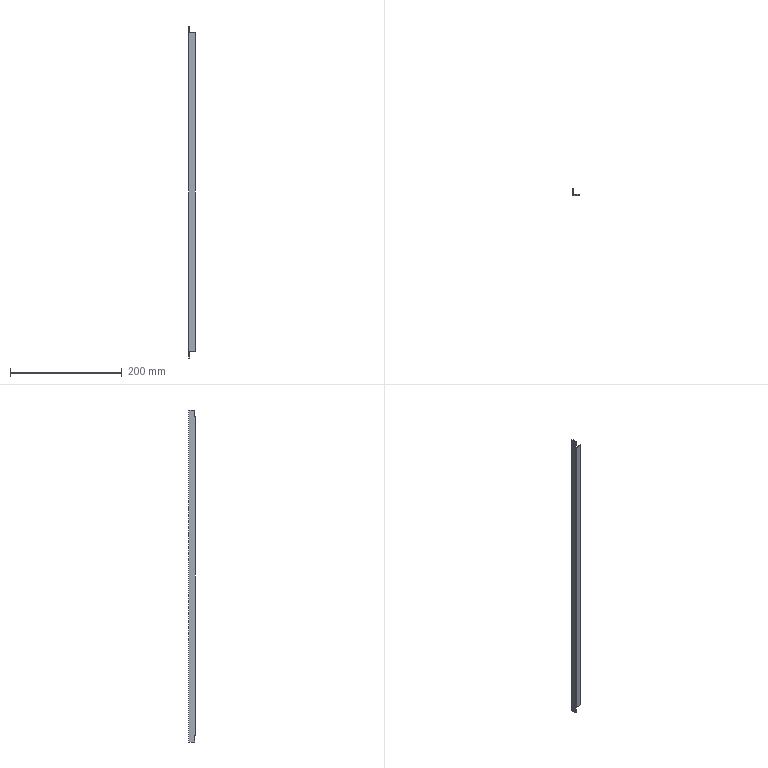Part | SolidWorks | features BaseBody 1 | 1 solid | 18 faces | box 12 x 12 x 594.4 mm | volume 15859 mm3 | plane 12 | cylinder 6 | commonest cylinder face diameters 0.6 x4 1 x2
STEP:
#1=CARTESIAN_POINT('',(0.,0.5,-284.7));
#2=VERTEX_POINT('',#1);
#3=CARTESIAN_POINT('',(0.5,0.,-284.7));
#4=VERTEX_POINT('',#3);
#5=CARTESIAN_POINT('',(0.5,0.5,-284.7));
#6=DIRECTION('',(0.,0.,1.));
#7=DIRECTION('',(-1.,0.,0.));
#8=AXIS2_PLACEMENT_3D('',#5,#6,#7);
#9=CIRCLE('',#8,0.5);
#10=EDGE_CURVE('',#2,#4,#9,.T.);
#11=ORIENTED_EDGE('',*,*,#10,.T.);
#12=CARTESIAN_POINT('',(0.5,0.,284.7));
#13=VERTEX_POINT('',#12);
#14=CARTESIAN_POINT('',(0.5,0.,0.));
#15=DIRECTION('',(0.,0.,-1.));
#16=VECTOR('',#15,1000.);
#17=LINE('',#14,#16);
#18=EDGE_CURVE('',#13,#4,#17,.T.);
#19=ORIENTED_EDGE('',*,*,#18,.F.);
#20=CARTESIAN_POINT('',(0.,0.5,284.7));
#21=VERTEX_POINT('',#20);
#22=CARTESIAN_POINT('',(0.5,0.5,284.7));
#23=DIRECTION('',(0.,0.,-1.));
#24=DIRECTION('',(-1.,0.,0.));
#25=AXIS2_PLACEMENT_3D('',#22,#23,#24);
#26=CIRCLE('',#25,0.5);
#27=EDGE_CURVE('',#13,#21,#26,.T.);
#28=ORIENTED_EDGE('',*,*,#27,.T.);
#29=CARTESIAN_POINT('',(0.,0.5,0.));
#30=DIRECTION('',(0.,0.,1.));
#31=VECTOR('',#30,1000.);
#32=LINE('',#29,#31);
#33=EDGE_CURVE('',#2,#21,#32,.T.);
#34=ORIENTED_EDGE('',*,*,#33,.F.);
#35=EDGE_LOOP('',(#11,#19,#28,#34));
#36=FACE_OUTER_BOUND('',#35,.T.);
#37=CARTESIAN_POINT('',(0.5,0.5,284.7));
#38=DIRECTION('',(0.,0.,-1.));
#39=DIRECTION('',(-1.,0.,0.));
#40=AXIS2_PLACEMENT_3D('',#37,#38,#39);
#41=CYLINDRICAL_SURFACE('',#40,0.5);
#42=ADVANCED_FACE('',(#36),#41,.T.);
#43=CARTESIAN_POINT('',(0.,1.2,-284.7));
#44=VERTEX_POINT('',#43);
#45=CARTESIAN_POINT('',(0.,0.6,-284.7));
#46=DIRECTION('',(0.,-1.,0.));
#47=VECTOR('',#46,1000.);
#48=LINE('',#45,#47);
#49=EDGE_CURVE('',#44,#2,#48,.T.);
#50=ORIENTED_EDGE('',*,*,#49,.T.);
#51=ORIENTED_EDGE('',*,*,#33,.T.);
#52=CARTESIAN_POINT('',(0.,1.2,284.7));
#53=VERTEX_POINT('',#52);
#54=CARTESIAN_POINT('',(0.,0.6,284.7));
#55=DIRECTION('',(0.,1.,0.));
#56=VECTOR('',#55,1000.);
#57=LINE('',#54,#56);
#58=EDGE_CURVE('',#21,#53,#57,.T.);
#59=ORIENTED_EDGE('',*,*,#58,.T.);
#60=CARTESIAN_POINT('',(0.,1.2,297.2));
#61=VERTEX_POINT('',#60);
#62=CARTESIAN_POINT('',(0.,1.2,0.));
#63=DIRECTION('',(0.,0.,-1.));
#64=VECTOR('',#63,1000.);
#65=LINE('',#62,#64);
#66=EDGE_CURVE('',#61,#53,#65,.T.);
#67=ORIENTED_EDGE('',*,*,#66,.F.);
#68=CARTESIAN_POINT('',(0.,11.7,297.2));
#69=VERTEX_POINT('',#68);
#70=CARTESIAN_POINT('',(0.,6.1,297.2));
#71=DIRECTION('',(0.,-1.,0.));
#72=VECTOR('',#71,1000.);
#73=LINE('',#70,#72);
#74=EDGE_CURVE('',#69,#61,#73,.T.);
#75=ORIENTED_EDGE('',*,*,#74,.F.);
#76=CARTESIAN_POINT('',(0.,11.7,-297.2));
#77=VERTEX_POINT('',#76);
#78=CARTESIAN_POINT('',(0.,11.7,0.));
#79=DIRECTION('',(0.,0.,1.));
#80=VECTOR('',#79,1000.);
#81=LINE('',#78,#80);
#82=EDGE_CURVE('',#77,#69,#81,.T.);
#83=ORIENTED_EDGE('',*,*,#82,.F.);
#84=CARTESIAN_POINT('',(0.,1.2,-297.2));
#85=VERTEX_POINT('',#84);
#86=CARTESIAN_POINT('',(0.,6.1,-297.2));
#87=DIRECTION('',(0.,1.,0.));
#88=VECTOR('',#87,1000.);
#89=LINE('',#86,#88);
#90=EDGE_CURVE('',#85,#77,#89,.T.);
#91=ORIENTED_EDGE('',*,*,#90,.F.);
#92=CARTESIAN_POINT('',(0.,1.2,0.));
#93=DIRECTION('',(0.,0.,-1.));
#94=VECTOR('',#93,1000.);
#95=LINE('',#92,#94);
#96=EDGE_CURVE('',#44,#85,#95,.T.);
#97=ORIENTED_EDGE('',*,*,#96,.F.);
#98=EDGE_LOOP('',(#50,#51,#59,#67,#75,#83,#91,#97));
#99=FACE_OUTER_BOUND('',#98,.T.);
#100=CARTESIAN_POINT('',(0.,0.5,297.2));
#101=DIRECTION('',(1.,0.,0.));
#102=DIRECTION('',(0.,0.,-1.));
#103=AXIS2_PLACEMENT_3D('',#100,#101,#102);
#104=PLANE('',#103);
#105=ADVANCED_FACE('',(#99),#104,.F.);
#106=CARTESIAN_POINT('',(11.7,0.,-284.7));
#107=VERTEX_POINT('',#106);
#108=CARTESIAN_POINT('',(6.1,0.,-284.7));
#109=DIRECTION('',(-1.,0.,0.));
#110=VECTOR('',#109,1000.);
#111=LINE('',#108,#110);
#112=EDGE_CURVE('',#107,#4,#111,.T.);
#113=ORIENTED_EDGE('',*,*,#112,.F.);
#114=CARTESIAN_POINT('',(11.7,0.,284.7));
#115=VERTEX_POINT('',#114);
#116=CARTESIAN_POINT('',(11.7,0.,0.));
#117=DIRECTION('',(0.,0.,-1.));
#118=VECTOR('',#117,1000.);
#119=LINE('',#116,#118);
#120=EDGE_CURVE('',#115,#107,#119,.T.);
#121=ORIENTED_EDGE('',*,*,#120,.F.);
#122=CARTESIAN_POINT('',(6.1,0.,284.7));
#123=DIRECTION('',(1.,0.,0.));
#124=VECTOR('',#123,1000.);
#125=LINE('',#122,#124);
#126=EDGE_CURVE('',#13,#115,#125,.T.);
#127=ORIENTED_EDGE('',*,*,#126,.F.);
#128=ORIENTED_EDGE('',*,*,#18,.T.);
#129=EDGE_LOOP('',(#113,#121,#127,#128));
#130=FACE_OUTER_BOUND('',#129,.T.);
#131=CARTESIAN_POINT('',(0.5,0.,-284.7));
#132=DIRECTION('',(0.,1.,0.));
#133=DIRECTION('',(0.,0.,1.));
#134=AXIS2_PLACEMENT_3D('',#131,#132,#133);
#135=PLANE('',#134);
#136=ADVANCED_FACE('',(#130),#135,.F.);
#137=CARTESIAN_POINT('',(1.7,1.2,-284.7));
#138=VERTEX_POINT('',#137);
#139=CARTESIAN_POINT('',(0.85,1.2,-284.7));
#140=DIRECTION('',(1.,0.,0.));
#141=VECTOR('',#140,1000.);
#142=LINE('',#139,#141);
#143=EDGE_CURVE('',#44,#138,#142,.T.);
#144=ORIENTED_EDGE('',*,*,#143,.F.);
#145=ORIENTED_EDGE('',*,*,#96,.T.);
#146=CARTESIAN_POINT('',(1.7,1.2,-297.2));
#147=VERTEX_POINT('',#146);
#148=CARTESIAN_POINT('',(0.85,1.2,-297.2));
#149=DIRECTION('',(-1.,0.,0.));
#150=VECTOR('',#149,1000.);
#151=LINE('',#148,#150);
#152=EDGE_CURVE('',#147,#85,#151,.T.);
#153=ORIENTED_EDGE('',*,*,#152,.F.);
#154=CARTESIAN_POINT('',(1.7,1.2,-290.95));
#155=DIRECTION('',(0.,0.,-1.));
#156=VECTOR('',#155,1000.);
#157=LINE('',#154,#156);
#158=EDGE_CURVE('',#138,#147,#157,.T.);
#159=ORIENTED_EDGE('',*,*,#158,.F.);
#160=EDGE_LOOP('',(#144,#145,#153,#159));
#161=FACE_OUTER_BOUND('',#160,.T.);
#162=CARTESIAN_POINT('',(0.,1.2,-297.2));
#163=DIRECTION('',(0.,1.,0.));
#164=DIRECTION('',(0.,0.,1.));
#165=AXIS2_PLACEMENT_3D('',#162,#163,#164);
#166=PLANE('',#165);
#167=ADVANCED_FACE('',(#161),#166,.F.);
#168=CARTESIAN_POINT('',(1.7,1.2,297.2));
#169=VERTEX_POINT('',#168);
#170=CARTESIAN_POINT('',(0.85,1.2,297.2));
#171=DIRECTION('',(1.,0.,0.));
#172=VECTOR('',#171,1000.);
#173=LINE('',#170,#172);
#174=EDGE_CURVE('',#61,#169,#173,.T.);
#175=ORIENTED_EDGE('',*,*,#174,.F.);
#176=ORIENTED_EDGE('',*,*,#66,.T.);
#177=CARTESIAN_POINT('',(1.7,1.2,284.7));
#178=VERTEX_POINT('',#177);
#179=CARTESIAN_POINT('',(0.85,1.2,284.7));
#180=DIRECTION('',(-1.,0.,0.));
#181=VECTOR('',#180,1000.);
#182=LINE('',#179,#181);
#183=EDGE_CURVE('',#178,#53,#182,.T.);
#184=ORIENTED_EDGE('',*,*,#183,.F.);
#185=CARTESIAN_POINT('',(1.7,1.2,290.95));
#186=DIRECTION('',(0.,0.,-1.));
#187=VECTOR('',#186,1000.);
#188=LINE('',#185,#187);
#189=EDGE_CURVE('',#169,#178,#188,.T.);
#190=ORIENTED_EDGE('',*,*,#189,.F.);
#191=EDGE_LOOP('',(#175,#176,#184,#190));
#192=FACE_OUTER_BOUND('',#191,.T.);
#193=CARTESIAN_POINT('',(0.,1.2,284.7));
#194=DIRECTION('',(0.,1.,0.));
#195=DIRECTION('',(0.,0.,1.));
#196=AXIS2_PLACEMENT_3D('',#193,#194,#195);
#197=PLANE('',#196);
#198=ADVANCED_FACE('',(#192),#197,.F.);
#199=ORIENTED_EDGE('',*,*,#174,.T.);
#200=CARTESIAN_POINT('',(1.2,1.7,297.2));
#201=VERTEX_POINT('',#200);
#202=CARTESIAN_POINT('',(1.7,1.7,297.2));
#203=DIRECTION('',(0.,0.,1.));
#204=DIRECTION('',(-1.,0.,0.));
#205=AXIS2_PLACEMENT_3D('',#202,#203,#204);
#206=CIRCLE('',#205,0.5);
#207=EDGE_CURVE('',#201,#169,#206,.T.);
#208=ORIENTED_EDGE('',*,*,#207,.F.);
#209=CARTESIAN_POINT('',(1.2,11.7,297.2));
#210=VERTEX_POINT('',#209);
#211=CARTESIAN_POINT('',(1.2,6.6,297.2));
#212=DIRECTION('',(0.,-1.,0.));
#213=VECTOR('',#212,1000.);
#214=LINE('',#211,#213);
#215=EDGE_CURVE('',#210,#201,#214,.T.);
#216=ORIENTED_EDGE('',*,*,#215,.F.);
#217=CARTESIAN_POINT('',(0.9,12.,297.2));
#218=VERTEX_POINT('',#217);
#219=CARTESIAN_POINT('',(0.9,11.7,297.2));
#220=DIRECTION('',(0.,0.,1.));
#221=DIRECTION('',(-1.,0.,0.));
#222=AXIS2_PLACEMENT_3D('',#219,#220,#221);
#223=CIRCLE('',#222,0.3);
#224=EDGE_CURVE('',#210,#218,#223,.T.);
#225=ORIENTED_EDGE('',*,*,#224,.T.);
#226=CARTESIAN_POINT('',(0.3,12.,297.2));
#227=VERTEX_POINT('',#226);
#228=CARTESIAN_POINT('',(0.6,12.,297.2));
#229=DIRECTION('',(-1.,0.,0.));
#230=VECTOR('',#229,1000.);
#231=LINE('',#228,#230);
#232=EDGE_CURVE('',#218,#227,#231,.T.);
#233=ORIENTED_EDGE('',*,*,#232,.T.);
#234=CARTESIAN_POINT('',(0.3,11.7,297.2));
#235=DIRECTION('',(0.,0.,-1.));
#236=DIRECTION('',(-1.,0.,0.));
#237=AXIS2_PLACEMENT_3D('',#234,#235,#236);
#238=CIRCLE('',#237,0.3);
#239=EDGE_CURVE('',#69,#227,#238,.T.);
#240=ORIENTED_EDGE('',*,*,#239,.F.);
#241=ORIENTED_EDGE('',*,*,#74,.T.);
#242=EDGE_LOOP('',(#199,#208,#216,#225,#233,#240,#241));
#243=FACE_OUTER_BOUND('',#242,.T.);
#244=CARTESIAN_POINT('',(1.71,1.2,297.2));
#245=DIRECTION('',(0.,0.,-1.));
#246=DIRECTION('',(-1.,0.,0.));
#247=AXIS2_PLACEMENT_3D('',#244,#245,#246);
#248=PLANE('',#247);
#249=ADVANCED_FACE('',(#243),#248,.F.);
#250=ORIENTED_EDGE('',*,*,#82,.T.);
#251=ORIENTED_EDGE('',*,*,#239,.T.);
#252=CARTESIAN_POINT('',(0.3,12.,-297.2));
#253=VERTEX_POINT('',#252);
#254=CARTESIAN_POINT('',(0.3,12.,0.));
#255=DIRECTION('',(0.,0.,1.));
#256=VECTOR('',#255,1000.);
#257=LINE('',#254,#256);
#258=EDGE_CURVE('',#253,#227,#257,.T.);
#259=ORIENTED_EDGE('',*,*,#258,.F.);
#260=CARTESIAN_POINT('',(0.3,11.7,-297.2));
#261=DIRECTION('',(0.,0.,-1.));
#262=DIRECTION('',(-1.,0.,0.));
#263=AXIS2_PLACEMENT_3D('',#260,#261,#262);
#264=CIRCLE('',#263,0.3);
#265=EDGE_CURVE('',#77,#253,#264,.T.);
#266=ORIENTED_EDGE('',*,*,#265,.F.);
#267=EDGE_LOOP('',(#250,#251,#259,#266));
#268=FACE_OUTER_BOUND('',#267,.T.);
#269=CARTESIAN_POINT('',(0.3,11.7,297.2));
#270=DIRECTION('',(0.,0.,-1.));
#271=DIRECTION('',(-1.,0.,0.));
#272=AXIS2_PLACEMENT_3D('',#269,#270,#271);
#273=CYLINDRICAL_SURFACE('',#272,0.3);
#274=ADVANCED_FACE('',(#268),#273,.T.);
#275=CARTESIAN_POINT('',(1.2,11.7,-297.2));
#276=VERTEX_POINT('',#275);
#277=CARTESIAN_POINT('',(1.2,1.7,-297.2));
#278=VERTEX_POINT('',#277);
#279=CARTESIAN_POINT('',(1.2,6.6,-297.2));
#280=DIRECTION('',(0.,-1.,0.));
#281=VECTOR('',#280,1000.);
#282=LINE('',#279,#281);
#283=EDGE_CURVE('',#276,#278,#282,.T.);
#284=ORIENTED_EDGE('',*,*,#283,.T.);
#285=CARTESIAN_POINT('',(1.7,1.7,-297.2));
#286=DIRECTION('',(0.,0.,1.));
#287=DIRECTION('',(-1.,0.,0.));
#288=AXIS2_PLACEMENT_3D('',#285,#286,#287);
#289=CIRCLE('',#288,0.5);
#290=EDGE_CURVE('',#278,#147,#289,.T.);
#291=ORIENTED_EDGE('',*,*,#290,.T.);
#292=ORIENTED_EDGE('',*,*,#152,.T.);
#293=ORIENTED_EDGE('',*,*,#90,.T.);
#294=ORIENTED_EDGE('',*,*,#265,.T.);
#295=CARTESIAN_POINT('',(0.9,12.,-297.2));
#296=VERTEX_POINT('',#295);
#297=CARTESIAN_POINT('',(0.8551,12.,-297.2));
#298=DIRECTION('',(1.,0.,0.));
#299=VECTOR('',#298,1000.);
#300=LINE('',#297,#299);
#301=EDGE_CURVE('',#253,#296,#300,.T.);
#302=ORIENTED_EDGE('',*,*,#301,.T.);
#303=CARTESIAN_POINT('',(0.9,11.7,-297.2));
#304=DIRECTION('',(0.,0.,-1.));
#305=DIRECTION('',(-1.,0.,0.));
#306=AXIS2_PLACEMENT_3D('',#303,#304,#305);
#307=CIRCLE('',#306,0.3);
#308=EDGE_CURVE('',#296,#276,#307,.T.);
#309=ORIENTED_EDGE('',*,*,#308,.T.);
#310=EDGE_LOOP('',(#284,#291,#292,#293,#294,#302,#309));
#311=FACE_OUTER_BOUND('',#310,.T.);
#312=CARTESIAN_POINT('',(1.71,1.2,-297.2));
#313=DIRECTION('',(0.,0.,-1.));
#314=DIRECTION('',(-1.,0.,0.));
#315=AXIS2_PLACEMENT_3D('',#312,#313,#314);
#316=PLANE('',#315);
#317=ADVANCED_FACE('',(#311),#316,.T.);
#318=ORIENTED_EDGE('',*,*,#10,.F.);
#319=ORIENTED_EDGE('',*,*,#49,.F.);
#320=ORIENTED_EDGE('',*,*,#143,.T.);
#321=CARTESIAN_POINT('',(11.7,1.2,-284.7));
#322=VERTEX_POINT('',#321);
#323=CARTESIAN_POINT('',(6.,1.2,-284.7));
#324=DIRECTION('',(-1.,0.,0.));
#325=VECTOR('',#324,1000.);
#326=LINE('',#323,#325);
#327=EDGE_CURVE('',#322,#138,#326,.T.);
#328=ORIENTED_EDGE('',*,*,#327,.F.);
#329=CARTESIAN_POINT('',(12.,0.9,-284.7));
#330=VERTEX_POINT('',#329);
#331=CARTESIAN_POINT('',(11.7,0.9,-284.7));
#332=DIRECTION('',(0.,0.,-1.));
#333=DIRECTION('',(-1.,0.,0.));
#334=AXIS2_PLACEMENT_3D('',#331,#332,#333);
#335=CIRCLE('',#334,0.3);
#336=EDGE_CURVE('',#322,#330,#335,.T.);
#337=ORIENTED_EDGE('',*,*,#336,.T.);
#338=CARTESIAN_POINT('',(12.,0.3,-284.7));
#339=VERTEX_POINT('',#338);
#340=CARTESIAN_POINT('',(12.,0.6,-284.7));
#341=DIRECTION('',(0.,-1.,0.));
#342=VECTOR('',#341,1000.);
#343=LINE('',#340,#342);
#344=EDGE_CURVE('',#330,#339,#343,.T.);
#345=ORIENTED_EDGE('',*,*,#344,.T.);
#346=CARTESIAN_POINT('',(11.7,0.3,-284.7));
#347=DIRECTION('',(0.,0.,1.));
#348=DIRECTION('',(-1.,0.,0.));
#349=AXIS2_PLACEMENT_3D('',#346,#347,#348);
#350=CIRCLE('',#349,0.3);
#351=EDGE_CURVE('',#107,#339,#350,.T.);
#352=ORIENTED_EDGE('',*,*,#351,.F.);
#353=ORIENTED_EDGE('',*,*,#112,.T.);
#354=EDGE_LOOP('',(#318,#319,#320,#328,#337,#345,#352,#353));
#355=FACE_OUTER_BOUND('',#354,.T.);
#356=CARTESIAN_POINT('',(0.,1.2,-284.7));
#357=DIRECTION('',(0.,0.,1.));
#358=DIRECTION('',(0.,-1.,0.));
#359=AXIS2_PLACEMENT_3D('',#356,#357,#358);
#360=PLANE('',#359);
#361=ADVANCED_FACE('',(#355),#360,.F.);
#362=ORIENTED_EDGE('',*,*,#351,.T.);
#363=CARTESIAN_POINT('',(12.,0.3,284.7));
#364=VERTEX_POINT('',#363);
#365=CARTESIAN_POINT('',(12.,0.3,0.));
#366=DIRECTION('',(0.,0.,-1.));
#367=VECTOR('',#366,1000.);
#368=LINE('',#365,#367);
#369=EDGE_CURVE('',#364,#339,#368,.T.);
#370=ORIENTED_EDGE('',*,*,#369,.F.);
#371=CARTESIAN_POINT('',(11.7,0.3,284.7));
#372=DIRECTION('',(0.,0.,1.));
#373=DIRECTION('',(-1.,0.,0.));
#374=AXIS2_PLACEMENT_3D('',#371,#372,#373);
#375=CIRCLE('',#374,0.3);
#376=EDGE_CURVE('',#115,#364,#375,.T.);
#377=ORIENTED_EDGE('',*,*,#376,.F.);
#378=ORIENTED_EDGE('',*,*,#120,.T.);
#379=EDGE_LOOP('',(#362,#370,#377,#378));
#380=FACE_OUTER_BOUND('',#379,.T.);
#381=CARTESIAN_POINT('',(11.7,0.3,284.7));
#382=DIRECTION('',(0.,0.,-1.));
#383=DIRECTION('',(-1.,0.,0.));
#384=AXIS2_PLACEMENT_3D('',#381,#382,#383);
#385=CYLINDRICAL_SURFACE('',#384,0.3);
#386=ADVANCED_FACE('',(#380),#385,.T.);
#387=CARTESIAN_POINT('',(12.,0.9,284.7));
#388=VERTEX_POINT('',#387);
#389=CARTESIAN_POINT('',(11.7,1.2,284.7));
#390=VERTEX_POINT('',#389);
#391=CARTESIAN_POINT('',(11.7,0.9,284.7));
#392=DIRECTION('',(0.,0.,1.));
#393=DIRECTION('',(-1.,0.,0.));
#394=AXIS2_PLACEMENT_3D('',#391,#392,#393);
#395=CIRCLE('',#394,0.3);
#396=EDGE_CURVE('',#388,#390,#395,.T.);
#397=ORIENTED_EDGE('',*,*,#396,.T.);
#398=CARTESIAN_POINT('',(6.,1.2,284.7));
#399=DIRECTION('',(1.,0.,0.));
#400=VECTOR('',#399,1000.);
#401=LINE('',#398,#400);
#402=EDGE_CURVE('',#178,#390,#401,.T.);
#403=ORIENTED_EDGE('',*,*,#402,.F.);
#404=ORIENTED_EDGE('',*,*,#183,.T.);
#405=ORIENTED_EDGE('',*,*,#58,.F.);
#406=ORIENTED_EDGE('',*,*,#27,.F.);
#407=ORIENTED_EDGE('',*,*,#126,.T.);
#408=ORIENTED_EDGE('',*,*,#376,.T.);
#409=CARTESIAN_POINT('',(12.,0.6,284.7));
#410=DIRECTION('',(0.,-1.,0.));
#411=VECTOR('',#410,1000.);
#412=LINE('',#409,#411);
#413=EDGE_CURVE('',#388,#364,#412,.T.);
#414=ORIENTED_EDGE('',*,*,#413,.F.);
#415=EDGE_LOOP('',(#397,#403,#404,#405,#406,#407,#408,#414));
#416=FACE_OUTER_BOUND('',#415,.T.);
#417=CARTESIAN_POINT('',(12.,0.,284.7));
#418=DIRECTION('',(0.,0.,-1.));
#419=DIRECTION('',(-1.,0.,0.));
#420=AXIS2_PLACEMENT_3D('',#417,#418,#419);
#421=PLANE('',#420);
#422=ADVANCED_FACE('',(#416),#421,.F.);
#423=CARTESIAN_POINT('',(1.7,1.2,0.));
#424=DIRECTION('',(0.,0.,-1.));
#425=VECTOR('',#424,1000.);
#426=LINE('',#423,#425);
#427=EDGE_CURVE('',#178,#138,#426,.T.);
#428=ORIENTED_EDGE('',*,*,#427,.T.);
#429=ORIENTED_EDGE('',*,*,#158,.T.);
#430=ORIENTED_EDGE('',*,*,#290,.F.);
#431=CARTESIAN_POINT('',(1.2,1.7,0.));
#432=DIRECTION('',(0.,0.,1.));
#433=VECTOR('',#432,1000.);
#434=LINE('',#431,#433);
#435=EDGE_CURVE('',#278,#201,#434,.T.);
#436=ORIENTED_EDGE('',*,*,#435,.T.);
#437=ORIENTED_EDGE('',*,*,#207,.T.);
#438=ORIENTED_EDGE('',*,*,#189,.T.);
#439=EDGE_LOOP('',(#428,#429,#430,#436,#437,#438));
#440=FACE_OUTER_BOUND('',#439,.T.);
#441=CARTESIAN_POINT('',(1.7,1.7,297.2));
#442=DIRECTION('',(0.,0.,-1.));
#443=DIRECTION('',(-1.,0.,0.));
#444=AXIS2_PLACEMENT_3D('',#441,#442,#443);
#445=CYLINDRICAL_SURFACE('',#444,0.5);
#446=ADVANCED_FACE('',(#440),#445,.F.);
#447=CARTESIAN_POINT('',(1.2,11.7,0.));
#448=DIRECTION('',(0.,0.,-1.));
#449=VECTOR('',#448,1000.);
#450=LINE('',#447,#449);
#451=EDGE_CURVE('',#210,#276,#450,.T.);
#452=ORIENTED_EDGE('',*,*,#451,.F.);
#453=ORIENTED_EDGE('',*,*,#215,.T.);
#454=ORIENTED_EDGE('',*,*,#435,.F.);
#455=ORIENTED_EDGE('',*,*,#283,.F.);
#456=EDGE_LOOP('',(#452,#453,#454,#455));
#457=FACE_OUTER_BOUND('',#456,.T.);
#458=CARTESIAN_POINT('',(1.2,11.7,-297.2));
#459=DIRECTION('',(-1.,0.,0.));
#460=DIRECTION('',(0.,-1.,0.));
#461=AXIS2_PLACEMENT_3D('',#458,#459,#460);
#462=PLANE('',#461);
#463=ADVANCED_FACE('',(#457),#462,.F.);
#464=ORIENTED_EDGE('',*,*,#258,.T.);
#465=ORIENTED_EDGE('',*,*,#232,.F.);
#466=CARTESIAN_POINT('',(0.9,12.,0.));
#467=DIRECTION('',(0.,0.,1.));
#468=VECTOR('',#467,1000.);
#469=LINE('',#466,#468);
#470=EDGE_CURVE('',#296,#218,#469,.T.);
#471=ORIENTED_EDGE('',*,*,#470,.F.);
#472=ORIENTED_EDGE('',*,*,#301,.F.);
#473=EDGE_LOOP('',(#464,#465,#471,#472));
#474=FACE_OUTER_BOUND('',#473,.T.);
#475=CARTESIAN_POINT('',(0.3,12.,297.2));
#476=DIRECTION('',(0.,-1.,0.));
#477=DIRECTION('',(0.,0.,-1.));
#478=AXIS2_PLACEMENT_3D('',#475,#476,#477);
#479=PLANE('',#478);
#480=ADVANCED_FACE('',(#474),#479,.F.);
#481=ORIENTED_EDGE('',*,*,#327,.T.);
#482=ORIENTED_EDGE('',*,*,#427,.F.);
#483=ORIENTED_EDGE('',*,*,#402,.T.);
#484=CARTESIAN_POINT('',(11.7,1.2,0.));
#485=DIRECTION('',(0.,0.,1.));
#486=VECTOR('',#485,1000.);
#487=LINE('',#484,#486);
#488=EDGE_CURVE('',#322,#390,#487,.T.);
#489=ORIENTED_EDGE('',*,*,#488,.F.);
#490=EDGE_LOOP('',(#481,#482,#483,#489));
#491=FACE_OUTER_BOUND('',#490,.T.);
#492=CARTESIAN_POINT('',(1.7,1.2,-284.7));
#493=DIRECTION('',(0.,-1.,0.));
#494=DIRECTION('',(1.,0.,0.));
#495=AXIS2_PLACEMENT_3D('',#492,#493,#494);
#496=PLANE('',#495);
#497=ADVANCED_FACE('',(#491),#496,.F.);
#498=ORIENTED_EDGE('',*,*,#344,.F.);
#499=CARTESIAN_POINT('',(12.,0.9,0.));
#500=DIRECTION('',(0.,0.,-1.));
#501=VECTOR('',#500,1000.);
#502=LINE('',#499,#501);
#503=EDGE_CURVE('',#388,#330,#502,.T.);
#504=ORIENTED_EDGE('',*,*,#503,.F.);
#505=ORIENTED_EDGE('',*,*,#413,.T.);
#506=ORIENTED_EDGE('',*,*,#369,.T.);
#507=EDGE_LOOP('',(#498,#504,#505,#506));
#508=FACE_OUTER_BOUND('',#507,.T.);
#509=CARTESIAN_POINT('',(12.,0.3,-284.7));
#510=DIRECTION('',(-1.,0.,0.));
#511=DIRECTION('',(0.,0.,1.));
#512=AXIS2_PLACEMENT_3D('',#509,#510,#511);
#513=PLANE('',#512);
#514=ADVANCED_FACE('',(#508),#513,.F.);
#515=ORIENTED_EDGE('',*,*,#470,.T.);
#516=ORIENTED_EDGE('',*,*,#224,.F.);
#517=ORIENTED_EDGE('',*,*,#451,.T.);
#518=ORIENTED_EDGE('',*,*,#308,.F.);
#519=EDGE_LOOP('',(#515,#516,#517,#518));
#520=FACE_OUTER_BOUND('',#519,.T.);
#521=CARTESIAN_POINT('',(0.9,11.7,297.2));
#522=DIRECTION('',(0.,0.,-1.));
#523=DIRECTION('',(-1.,0.,0.));
#524=AXIS2_PLACEMENT_3D('',#521,#522,#523);
#525=CYLINDRICAL_SURFACE('',#524,0.3);
#526=ADVANCED_FACE('',(#520),#525,.T.);
#527=ORIENTED_EDGE('',*,*,#336,.F.);
#528=ORIENTED_EDGE('',*,*,#488,.T.);
#529=ORIENTED_EDGE('',*,*,#396,.F.);
#530=ORIENTED_EDGE('',*,*,#503,.T.);
#531=EDGE_LOOP('',(#527,#528,#529,#530));
#532=FACE_OUTER_BOUND('',#531,.T.);
#533=CARTESIAN_POINT('',(11.7,0.9,284.7));
#534=DIRECTION('',(0.,0.,-1.));
#535=DIRECTION('',(-1.,0.,0.));
#536=AXIS2_PLACEMENT_3D('',#533,#534,#535);
#537=CYLINDRICAL_SURFACE('',#536,0.3);
#538=ADVANCED_FACE('',(#532),#537,.T.);
#539=CLOSED_SHELL('',(#42,#105,#136,#167,#198,#249,#274,#317,#361,#386,#422,#446,#463,#480,#497,#514,#526,#538));
#540=MANIFOLD_SOLID_BREP('',#539);
#541=CARTESIAN_POINT('',(0.,0.,0.));
#542=DIRECTION('',(0.,0.,1.));
#543=DIRECTION('',(1.,0.,0.));
#544=AXIS2_PLACEMENT_3D('',#541,#542,#543);
#545=(LENGTH_UNIT()NAMED_UNIT(*)SI_UNIT(.MILLI.,.METRE.));
#546=UNCERTAINTY_MEASURE_WITH_UNIT(LENGTH_MEASURE(0.00001),#545,'','');
#547=(NAMED_UNIT(*)PLANE_ANGLE_UNIT()SI_UNIT($,.RADIAN.));
#548=(NAMED_UNIT(*)SI_UNIT($,.STERADIAN.)SOLID_ANGLE_UNIT());
#549=(GEOMETRIC_REPRESENTATION_CONTEXT(3)GLOBAL_UNCERTAINTY_ASSIGNED_CONTEXT((#546))GLOBAL_UNIT_ASSIGNED_CONTEXT((#545,#547,#548))REPRESENTATION_CONTEXT('',''));
#550=ADVANCED_BREP_SHAPE_REPRESENTATION('',(#540,#544),#549);